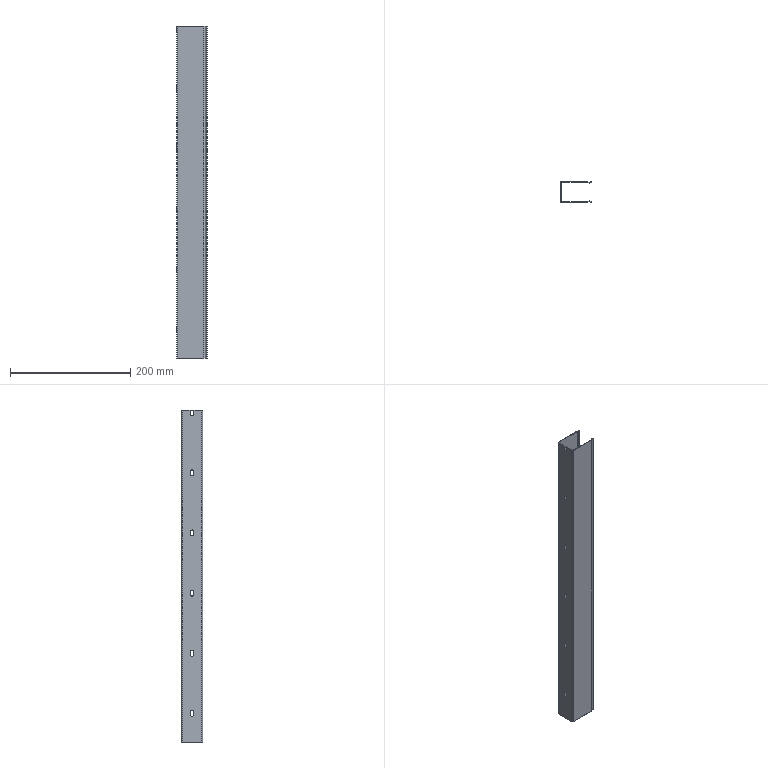Part | STEP file | 35 wire duct_552 | 1 solid | 53 faces | box 50.625 x 35 x 552 mm | volume 74720 mm3 | plane 31 | cylinder 22 | commonest cylinder face diameters 5 x18 1 x2 3 x2